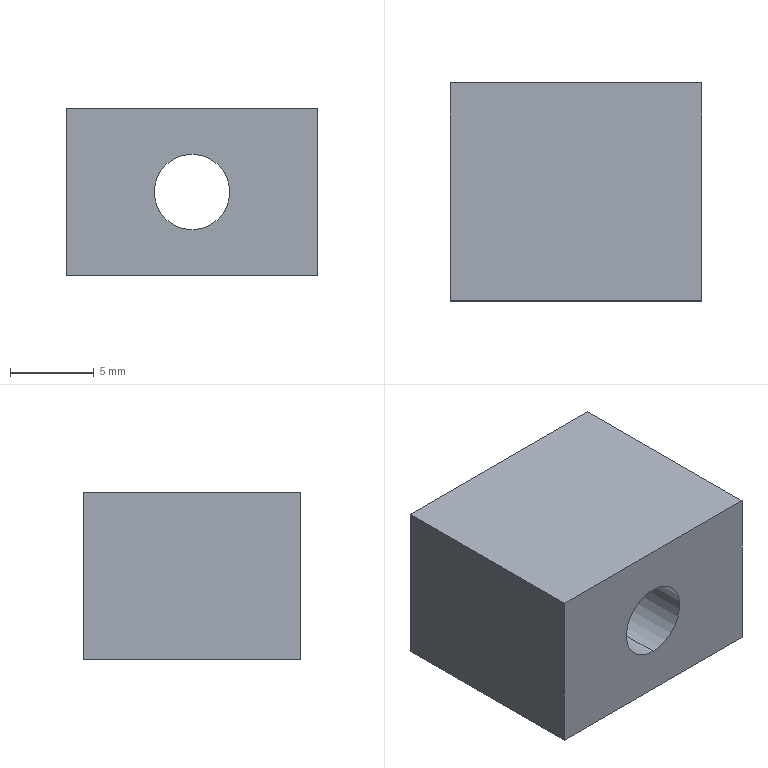Part | SolidWorks | features Extrusion 1, HoleWzd 1 | 1 solid | 11 faces | box 15 x 13 x 10 mm | volume 1585 mm3 | plane 7 | cylinder 4 | commonest cylinder face diameters 4.5 x2 8 x2
STEP:
#1=CARTESIAN_POINT('',(0.,1.9,-4.));
#2=VERTEX_POINT('',#1);
#3=CARTESIAN_POINT('',(0.,1.9,4.));
#4=VERTEX_POINT('',#3);
#5=CARTESIAN_POINT('',(0.,1.9,0.));
#6=DIRECTION('',(0.,1.,0.));
#7=DIRECTION('',(0.,0.,1.));
#8=AXIS2_PLACEMENT_3D('',#5,#6,#7);
#9=CIRCLE('',#8,4.);
#10=EDGE_CURVE('',#2,#4,#9,.T.);
#11=ORIENTED_EDGE('',*,*,#10,.F.);
#12=CARTESIAN_POINT('',(0.,6.5,-4.));
#13=VERTEX_POINT('',#12);
#14=CARTESIAN_POINT('',(0.,6.5,-4.));
#15=DIRECTION('',(0.,1.,0.));
#16=VECTOR('',#15,1000.);
#17=LINE('',#14,#16);
#18=EDGE_CURVE('',#2,#13,#17,.T.);
#19=ORIENTED_EDGE('',*,*,#18,.T.);
#20=CARTESIAN_POINT('',(0.,6.5,4.));
#21=VERTEX_POINT('',#20);
#22=CARTESIAN_POINT('',(0.,6.5,0.));
#23=DIRECTION('',(0.,1.,0.));
#24=DIRECTION('',(0.,0.,1.));
#25=AXIS2_PLACEMENT_3D('',#22,#23,#24);
#26=CIRCLE('',#25,4.);
#27=EDGE_CURVE('',#13,#21,#26,.T.);
#28=ORIENTED_EDGE('',*,*,#27,.T.);
#29=CARTESIAN_POINT('',(0.,6.5,4.));
#30=DIRECTION('',(0.,1.,0.));
#31=VECTOR('',#30,1000.);
#32=LINE('',#29,#31);
#33=EDGE_CURVE('',#4,#21,#32,.T.);
#34=ORIENTED_EDGE('',*,*,#33,.F.);
#35=EDGE_LOOP('',(#11,#19,#28,#34));
#36=FACE_OUTER_BOUND('',#35,.T.);
#37=CARTESIAN_POINT('',(0.,6.5,0.));
#38=DIRECTION('',(0.,1.,0.));
#39=DIRECTION('',(0.,0.,1.));
#40=AXIS2_PLACEMENT_3D('',#37,#38,#39);
#41=CYLINDRICAL_SURFACE('',#40,4.);
#42=ADVANCED_FACE('',(#36),#41,.F.);
#43=CARTESIAN_POINT('',(0.,-6.5,-2.25));
#44=VERTEX_POINT('',#43);
#45=CARTESIAN_POINT('',(0.,-6.5,2.25));
#46=VERTEX_POINT('',#45);
#47=CARTESIAN_POINT('',(0.,-6.5,0.));
#48=DIRECTION('',(0.,1.,0.));
#49=DIRECTION('',(0.,0.,1.));
#50=AXIS2_PLACEMENT_3D('',#47,#48,#49);
#51=CIRCLE('',#50,2.25);
#52=EDGE_CURVE('',#44,#46,#51,.T.);
#53=ORIENTED_EDGE('',*,*,#52,.F.);
#54=CARTESIAN_POINT('',(0.,1.9,-2.25));
#55=VERTEX_POINT('',#54);
#56=CARTESIAN_POINT('',(0.,6.5,-2.25));
#57=DIRECTION('',(0.,1.,0.));
#58=VECTOR('',#57,1000.);
#59=LINE('',#56,#58);
#60=EDGE_CURVE('',#44,#55,#59,.T.);
#61=ORIENTED_EDGE('',*,*,#60,.T.);
#62=CARTESIAN_POINT('',(0.,1.9,2.25));
#63=VERTEX_POINT('',#62);
#64=CARTESIAN_POINT('',(0.,1.9,0.));
#65=DIRECTION('',(0.,1.,0.));
#66=DIRECTION('',(0.,0.,1.));
#67=AXIS2_PLACEMENT_3D('',#64,#65,#66);
#68=CIRCLE('',#67,2.25);
#69=EDGE_CURVE('',#55,#63,#68,.T.);
#70=ORIENTED_EDGE('',*,*,#69,.T.);
#71=CARTESIAN_POINT('',(0.,6.5,2.25));
#72=DIRECTION('',(0.,1.,0.));
#73=VECTOR('',#72,1000.);
#74=LINE('',#71,#73);
#75=EDGE_CURVE('',#46,#63,#74,.T.);
#76=ORIENTED_EDGE('',*,*,#75,.F.);
#77=EDGE_LOOP('',(#53,#61,#70,#76));
#78=FACE_OUTER_BOUND('',#77,.T.);
#79=CARTESIAN_POINT('',(0.,6.5,0.));
#80=DIRECTION('',(0.,1.,0.));
#81=DIRECTION('',(0.,0.,1.));
#82=AXIS2_PLACEMENT_3D('',#79,#80,#81);
#83=CYLINDRICAL_SURFACE('',#82,2.25);
#84=ADVANCED_FACE('',(#78),#83,.F.);
#85=CARTESIAN_POINT('',(7.5,-6.5,5.));
#86=VERTEX_POINT('',#85);
#87=CARTESIAN_POINT('',(7.5,-6.5,-5.));
#88=VERTEX_POINT('',#87);
#89=CARTESIAN_POINT('',(7.5,-6.5,5.));
#90=DIRECTION('',(0.,0.,-1.));
#91=VECTOR('',#90,1000.);
#92=LINE('',#89,#91);
#93=EDGE_CURVE('',#86,#88,#92,.T.);
#94=ORIENTED_EDGE('',*,*,#93,.T.);
#95=CARTESIAN_POINT('',(7.5,6.5,-5.));
#96=VERTEX_POINT('',#95);
#97=CARTESIAN_POINT('',(7.5,6.5,-5.));
#98=DIRECTION('',(0.,-1.,0.));
#99=VECTOR('',#98,1000.);
#100=LINE('',#97,#99);
#101=EDGE_CURVE('',#96,#88,#100,.T.);
#102=ORIENTED_EDGE('',*,*,#101,.F.);
#103=CARTESIAN_POINT('',(7.5,6.5,5.));
#104=VERTEX_POINT('',#103);
#105=CARTESIAN_POINT('',(7.5,6.5,5.));
#106=DIRECTION('',(0.,0.,-1.));
#107=VECTOR('',#106,1000.);
#108=LINE('',#105,#107);
#109=EDGE_CURVE('',#104,#96,#108,.T.);
#110=ORIENTED_EDGE('',*,*,#109,.F.);
#111=CARTESIAN_POINT('',(7.5,6.5,5.));
#112=DIRECTION('',(0.,-1.,0.));
#113=VECTOR('',#112,1000.);
#114=LINE('',#111,#113);
#115=EDGE_CURVE('',#104,#86,#114,.T.);
#116=ORIENTED_EDGE('',*,*,#115,.T.);
#117=EDGE_LOOP('',(#94,#102,#110,#116));
#118=FACE_OUTER_BOUND('',#117,.T.);
#119=CARTESIAN_POINT('',(7.5,6.5,5.));
#120=DIRECTION('',(-1.,0.,0.));
#121=DIRECTION('',(0.,0.,1.));
#122=AXIS2_PLACEMENT_3D('',#119,#120,#121);
#123=PLANE('',#122);
#124=ADVANCED_FACE('',(#118),#123,.F.);
#125=CARTESIAN_POINT('',(-7.5,-6.5,-5.));
#126=VERTEX_POINT('',#125);
#127=CARTESIAN_POINT('',(-7.5,-6.5,-5.));
#128=DIRECTION('',(-1.,0.,0.));
#129=VECTOR('',#128,1000.);
#130=LINE('',#127,#129);
#131=EDGE_CURVE('',#88,#126,#130,.T.);
#132=ORIENTED_EDGE('',*,*,#131,.T.);
#133=CARTESIAN_POINT('',(-7.5,6.5,-5.));
#134=VERTEX_POINT('',#133);
#135=CARTESIAN_POINT('',(-7.5,6.5,-5.));
#136=DIRECTION('',(0.,-1.,0.));
#137=VECTOR('',#136,1000.);
#138=LINE('',#135,#137);
#139=EDGE_CURVE('',#134,#126,#138,.T.);
#140=ORIENTED_EDGE('',*,*,#139,.F.);
#141=CARTESIAN_POINT('',(-7.5,6.5,-5.));
#142=DIRECTION('',(-1.,0.,0.));
#143=VECTOR('',#142,1000.);
#144=LINE('',#141,#143);
#145=EDGE_CURVE('',#96,#134,#144,.T.);
#146=ORIENTED_EDGE('',*,*,#145,.F.);
#147=ORIENTED_EDGE('',*,*,#101,.T.);
#148=EDGE_LOOP('',(#132,#140,#146,#147));
#149=FACE_OUTER_BOUND('',#148,.T.);
#150=CARTESIAN_POINT('',(-7.5,6.5,-5.));
#151=DIRECTION('',(0.,0.,1.));
#152=DIRECTION('',(1.,0.,0.));
#153=AXIS2_PLACEMENT_3D('',#150,#151,#152);
#154=PLANE('',#153);
#155=ADVANCED_FACE('',(#149),#154,.F.);
#156=CARTESIAN_POINT('',(-7.5,-6.5,5.));
#157=VERTEX_POINT('',#156);
#158=CARTESIAN_POINT('',(-7.5,-6.5,5.));
#159=DIRECTION('',(0.,0.,1.));
#160=VECTOR('',#159,1000.);
#161=LINE('',#158,#160);
#162=EDGE_CURVE('',#126,#157,#161,.T.);
#163=ORIENTED_EDGE('',*,*,#162,.T.);
#164=CARTESIAN_POINT('',(-7.5,6.5,5.));
#165=VERTEX_POINT('',#164);
#166=CARTESIAN_POINT('',(-7.5,6.5,5.));
#167=DIRECTION('',(0.,-1.,0.));
#168=VECTOR('',#167,1000.);
#169=LINE('',#166,#168);
#170=EDGE_CURVE('',#165,#157,#169,.T.);
#171=ORIENTED_EDGE('',*,*,#170,.F.);
#172=CARTESIAN_POINT('',(-7.5,6.5,5.));
#173=DIRECTION('',(0.,0.,1.));
#174=VECTOR('',#173,1000.);
#175=LINE('',#172,#174);
#176=EDGE_CURVE('',#134,#165,#175,.T.);
#177=ORIENTED_EDGE('',*,*,#176,.F.);
#178=ORIENTED_EDGE('',*,*,#139,.T.);
#179=EDGE_LOOP('',(#163,#171,#177,#178));
#180=FACE_OUTER_BOUND('',#179,.T.);
#181=CARTESIAN_POINT('',(-7.5,6.5,5.));
#182=DIRECTION('',(1.,0.,0.));
#183=DIRECTION('',(0.,0.,-1.));
#184=AXIS2_PLACEMENT_3D('',#181,#182,#183);
#185=PLANE('',#184);
#186=ADVANCED_FACE('',(#180),#185,.F.);
#187=CARTESIAN_POINT('',(-7.5,-6.5,5.));
#188=DIRECTION('',(1.,0.,0.));
#189=VECTOR('',#188,1000.);
#190=LINE('',#187,#189);
#191=EDGE_CURVE('',#157,#86,#190,.T.);
#192=ORIENTED_EDGE('',*,*,#191,.T.);
#193=ORIENTED_EDGE('',*,*,#115,.F.);
#194=CARTESIAN_POINT('',(-7.5,6.5,5.));
#195=DIRECTION('',(1.,0.,0.));
#196=VECTOR('',#195,1000.);
#197=LINE('',#194,#196);
#198=EDGE_CURVE('',#165,#104,#197,.T.);
#199=ORIENTED_EDGE('',*,*,#198,.F.);
#200=ORIENTED_EDGE('',*,*,#170,.T.);
#201=EDGE_LOOP('',(#192,#193,#199,#200));
#202=FACE_OUTER_BOUND('',#201,.T.);
#203=CARTESIAN_POINT('',(-7.5,6.5,5.));
#204=DIRECTION('',(0.,0.,-1.));
#205=DIRECTION('',(-1.,0.,0.));
#206=AXIS2_PLACEMENT_3D('',#203,#204,#205);
#207=PLANE('',#206);
#208=ADVANCED_FACE('',(#202),#207,.F.);
#209=CARTESIAN_POINT('',(0.,6.5,0.));
#210=DIRECTION('',(0.,1.,0.));
#211=DIRECTION('',(0.,0.,1.));
#212=AXIS2_PLACEMENT_3D('',#209,#210,#211);
#213=CIRCLE('',#212,4.);
#214=EDGE_CURVE('',#21,#13,#213,.T.);
#215=ORIENTED_EDGE('',*,*,#214,.F.);
#216=ORIENTED_EDGE('',*,*,#27,.F.);
#217=EDGE_LOOP('',(#215,#216));
#218=FACE_BOUND('',#217,.T.);
#219=ORIENTED_EDGE('',*,*,#109,.T.);
#220=ORIENTED_EDGE('',*,*,#145,.T.);
#221=ORIENTED_EDGE('',*,*,#176,.T.);
#222=ORIENTED_EDGE('',*,*,#198,.T.);
#223=EDGE_LOOP('',(#219,#220,#221,#222));
#224=FACE_OUTER_BOUND('',#223,.T.);
#225=CARTESIAN_POINT('',(0.,6.5,0.));
#226=DIRECTION('',(0.,-1.,0.));
#227=DIRECTION('',(0.,0.,-1.));
#228=AXIS2_PLACEMENT_3D('',#225,#226,#227);
#229=PLANE('',#228);
#230=ADVANCED_FACE('',(#218,#224),#229,.F.);
#231=CARTESIAN_POINT('',(0.,-6.5,0.));
#232=DIRECTION('',(0.,1.,0.));
#233=DIRECTION('',(0.,0.,1.));
#234=AXIS2_PLACEMENT_3D('',#231,#232,#233);
#235=CIRCLE('',#234,2.25);
#236=EDGE_CURVE('',#46,#44,#235,.T.);
#237=ORIENTED_EDGE('',*,*,#236,.T.);
#238=ORIENTED_EDGE('',*,*,#52,.T.);
#239=EDGE_LOOP('',(#237,#238));
#240=FACE_BOUND('',#239,.T.);
#241=ORIENTED_EDGE('',*,*,#93,.F.);
#242=ORIENTED_EDGE('',*,*,#191,.F.);
#243=ORIENTED_EDGE('',*,*,#162,.F.);
#244=ORIENTED_EDGE('',*,*,#131,.F.);
#245=EDGE_LOOP('',(#241,#242,#243,#244));
#246=FACE_OUTER_BOUND('',#245,.T.);
#247=CARTESIAN_POINT('',(0.,-6.5,0.));
#248=DIRECTION('',(0.,-1.,0.));
#249=DIRECTION('',(0.,0.,-1.));
#250=AXIS2_PLACEMENT_3D('',#247,#248,#249);
#251=PLANE('',#250);
#252=ADVANCED_FACE('',(#240,#246),#251,.T.);
#253=ORIENTED_EDGE('',*,*,#60,.F.);
#254=ORIENTED_EDGE('',*,*,#236,.F.);
#255=ORIENTED_EDGE('',*,*,#75,.T.);
#256=CARTESIAN_POINT('',(0.,1.9,0.));
#257=DIRECTION('',(0.,1.,0.));
#258=DIRECTION('',(0.,0.,1.));
#259=AXIS2_PLACEMENT_3D('',#256,#257,#258);
#260=CIRCLE('',#259,2.25);
#261=EDGE_CURVE('',#63,#55,#260,.T.);
#262=ORIENTED_EDGE('',*,*,#261,.T.);
#263=EDGE_LOOP('',(#253,#254,#255,#262));
#264=FACE_OUTER_BOUND('',#263,.T.);
#265=CARTESIAN_POINT('',(0.,6.5,0.));
#266=DIRECTION('',(0.,1.,0.));
#267=DIRECTION('',(0.,0.,1.));
#268=AXIS2_PLACEMENT_3D('',#265,#266,#267);
#269=CYLINDRICAL_SURFACE('',#268,2.25);
#270=ADVANCED_FACE('',(#264),#269,.F.);
#271=ORIENTED_EDGE('',*,*,#261,.F.);
#272=ORIENTED_EDGE('',*,*,#69,.F.);
#273=EDGE_LOOP('',(#271,#272));
#274=FACE_BOUND('',#273,.T.);
#275=CARTESIAN_POINT('',(0.,1.9,0.));
#276=DIRECTION('',(0.,1.,0.));
#277=DIRECTION('',(0.,0.,1.));
#278=AXIS2_PLACEMENT_3D('',#275,#276,#277);
#279=CIRCLE('',#278,4.);
#280=EDGE_CURVE('',#4,#2,#279,.T.);
#281=ORIENTED_EDGE('',*,*,#280,.T.);
#282=ORIENTED_EDGE('',*,*,#10,.T.);
#283=EDGE_LOOP('',(#281,#282));
#284=FACE_OUTER_BOUND('',#283,.T.);
#285=CARTESIAN_POINT('',(2.25,1.9,0.));
#286=DIRECTION('',(0.,-1.,0.));
#287=DIRECTION('',(0.,0.,-1.));
#288=AXIS2_PLACEMENT_3D('',#285,#286,#287);
#289=PLANE('',#288);
#290=ADVANCED_FACE('',(#274,#284),#289,.F.);
#291=ORIENTED_EDGE('',*,*,#18,.F.);
#292=ORIENTED_EDGE('',*,*,#280,.F.);
#293=ORIENTED_EDGE('',*,*,#33,.T.);
#294=ORIENTED_EDGE('',*,*,#214,.T.);
#295=EDGE_LOOP('',(#291,#292,#293,#294));
#296=FACE_OUTER_BOUND('',#295,.T.);
#297=CARTESIAN_POINT('',(0.,6.5,0.));
#298=DIRECTION('',(0.,1.,0.));
#299=DIRECTION('',(0.,0.,1.));
#300=AXIS2_PLACEMENT_3D('',#297,#298,#299);
#301=CYLINDRICAL_SURFACE('',#300,4.);
#302=ADVANCED_FACE('',(#296),#301,.F.);
#303=CLOSED_SHELL('',(#42,#84,#124,#155,#186,#208,#230,#252,#270,#290,#302));
#304=MANIFOLD_SOLID_BREP('',#303);
#305=CARTESIAN_POINT('',(0.,0.,0.));
#306=DIRECTION('',(0.,0.,1.));
#307=DIRECTION('',(1.,0.,0.));
#308=AXIS2_PLACEMENT_3D('',#305,#306,#307);
#309=(LENGTH_UNIT()NAMED_UNIT(*)SI_UNIT(.MILLI.,.METRE.));
#310=UNCERTAINTY_MEASURE_WITH_UNIT(LENGTH_MEASURE(0.00001),#309,'','');
#311=(NAMED_UNIT(*)PLANE_ANGLE_UNIT()SI_UNIT($,.RADIAN.));
#312=(NAMED_UNIT(*)SI_UNIT($,.STERADIAN.)SOLID_ANGLE_UNIT());
#313=(GEOMETRIC_REPRESENTATION_CONTEXT(3)GLOBAL_UNCERTAINTY_ASSIGNED_CONTEXT((#310))GLOBAL_UNIT_ASSIGNED_CONTEXT((#309,#311,#312))REPRESENTATION_CONTEXT('',''));
#314=ADVANCED_BREP_SHAPE_REPRESENTATION('',(#304,#308),#313);